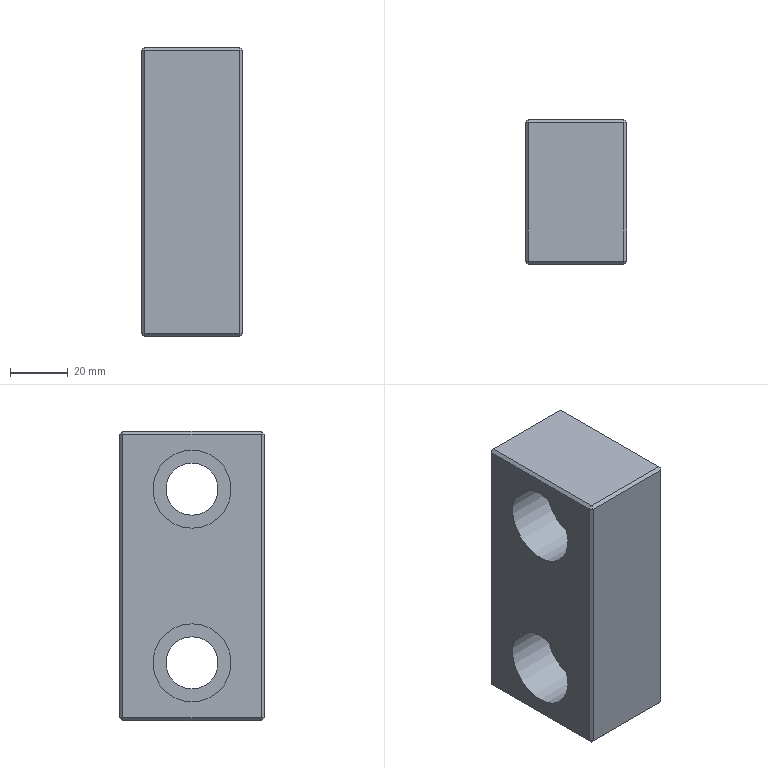Part | STEP file | 车灯-后视镜_id70_x_t | 1 solid | 32 faces | box 35 x 50 x 100 mm | volume 146008 mm3 | plane 28 | cylinder 4 | commonest cylinder face diameters 18 x2 27 x2
STEP:
#1=CARTESIAN_POINT('',(-284.,229.,49.5));
#2=VERTEX_POINT('',#1);
#3=CARTESIAN_POINT('',(-284.,181.,49.5));
#4=VERTEX_POINT('',#3);
#5=CARTESIAN_POINT('',(-284.,205.,49.5));
#6=DIRECTION('',(0.,-1.,0.));
#7=VECTOR('',#6,1.);
#8=LINE('',#5,#7);
#9=EDGE_CURVE('',#2,#4,#8,.T.);
#10=ORIENTED_EDGE('',*,*,#9,.T.);
#11=CARTESIAN_POINT('',(-251.,181.,49.5));
#12=VERTEX_POINT('',#11);
#13=CARTESIAN_POINT('',(-265.,181.,49.5));
#14=DIRECTION('',(1.,0.,0.));
#15=VECTOR('',#14,1.);
#16=LINE('',#13,#15);
#17=EDGE_CURVE('',#4,#12,#16,.T.);
#18=ORIENTED_EDGE('',*,*,#17,.T.);
#19=CARTESIAN_POINT('',(-251.,229.,49.5));
#20=VERTEX_POINT('',#19);
#21=CARTESIAN_POINT('',(-251.,205.,49.5));
#22=DIRECTION('',(0.,1.,0.));
#23=VECTOR('',#22,1.);
#24=LINE('',#21,#23);
#25=EDGE_CURVE('',#12,#20,#24,.T.);
#26=ORIENTED_EDGE('',*,*,#25,.T.);
#27=CARTESIAN_POINT('',(-265.,229.,49.5));
#28=DIRECTION('',(-1.,0.,0.));
#29=VECTOR('',#28,1.);
#30=LINE('',#27,#29);
#31=EDGE_CURVE('',#20,#2,#30,.T.);
#32=ORIENTED_EDGE('',*,*,#31,.T.);
#33=EDGE_LOOP('',(#10,#18,#26,#32));
#34=FACE_OUTER_BOUND('',#33,.T.);
#35=CARTESIAN_POINT('',(-265.,205.,49.5));
#36=DIRECTION('',(0.,0.,1.));
#37=DIRECTION('',(-1.,0.,0.));
#38=AXIS2_PLACEMENT_3D('',#35,#36,#37);
#39=PLANE('',#38);
#40=ADVANCED_FACE('',(#34),#39,.T.);
#41=CARTESIAN_POINT('',(-251.,230.,48.5));
#42=VERTEX_POINT('',#41);
#43=CARTESIAN_POINT('',(-251.,230.,-49.5));
#44=VERTEX_POINT('',#43);
#45=CARTESIAN_POINT('',(-251.,230.,-60.5));
#46=DIRECTION('',(0.,0.,-1.));
#47=VECTOR('',#46,1.);
#48=LINE('',#45,#47);
#49=EDGE_CURVE('',#42,#44,#48,.T.);
#50=ORIENTED_EDGE('',*,*,#49,.T.);
#51=CARTESIAN_POINT('',(-284.,230.,-49.5));
#52=VERTEX_POINT('',#51);
#53=CARTESIAN_POINT('',(-255.,230.,-49.5));
#54=DIRECTION('',(-1.,0.,0.));
#55=VECTOR('',#54,1.);
#56=LINE('',#53,#55);
#57=EDGE_CURVE('',#44,#52,#56,.T.);
#58=ORIENTED_EDGE('',*,*,#57,.T.);
#59=CARTESIAN_POINT('',(-284.,230.,48.5));
#60=VERTEX_POINT('',#59);
#61=CARTESIAN_POINT('',(-284.,230.,-60.5));
#62=DIRECTION('',(0.,0.,1.));
#63=VECTOR('',#62,1.);
#64=LINE('',#61,#63);
#65=EDGE_CURVE('',#52,#60,#64,.T.);
#66=ORIENTED_EDGE('',*,*,#65,.T.);
#67=CARTESIAN_POINT('',(-255.,230.,48.5));
#68=DIRECTION('',(1.,0.,0.));
#69=VECTOR('',#68,1.);
#70=LINE('',#67,#69);
#71=EDGE_CURVE('',#60,#42,#70,.T.);
#72=ORIENTED_EDGE('',*,*,#71,.T.);
#73=EDGE_LOOP('',(#50,#58,#66,#72));
#74=FACE_OUTER_BOUND('',#73,.T.);
#75=CARTESIAN_POINT('',(-255.,230.,-60.5));
#76=DIRECTION('',(0.,1.,0.));
#77=DIRECTION('',(0.,0.,-1.));
#78=AXIS2_PLACEMENT_3D('',#75,#76,#77);
#79=PLANE('',#78);
#80=ADVANCED_FACE('',(#74),#79,.T.);
#81=CARTESIAN_POINT('',(-250.,181.,48.5));
#82=VERTEX_POINT('',#81);
#83=CARTESIAN_POINT('',(-250.,181.,-49.5));
#84=VERTEX_POINT('',#83);
#85=CARTESIAN_POINT('',(-250.,181.,-60.5));
#86=DIRECTION('',(0.,0.,-1.));
#87=VECTOR('',#86,1.);
#88=LINE('',#85,#87);
#89=EDGE_CURVE('',#82,#84,#88,.T.);
#90=ORIENTED_EDGE('',*,*,#89,.T.);
#91=CARTESIAN_POINT('',(-250.,229.,-49.5));
#92=VERTEX_POINT('',#91);
#93=CARTESIAN_POINT('',(-250.,205.,-49.5));
#94=DIRECTION('',(0.,1.,0.));
#95=VECTOR('',#94,1.);
#96=LINE('',#93,#95);
#97=EDGE_CURVE('',#84,#92,#96,.T.);
#98=ORIENTED_EDGE('',*,*,#97,.T.);
#99=CARTESIAN_POINT('',(-250.,229.,48.5));
#100=VERTEX_POINT('',#99);
#101=CARTESIAN_POINT('',(-250.,229.,-60.5));
#102=DIRECTION('',(0.,0.,1.));
#103=VECTOR('',#102,1.);
#104=LINE('',#101,#103);
#105=EDGE_CURVE('',#92,#100,#104,.T.);
#106=ORIENTED_EDGE('',*,*,#105,.T.);
#107=CARTESIAN_POINT('',(-250.,205.,48.5));
#108=DIRECTION('',(0.,-1.,0.));
#109=VECTOR('',#108,1.);
#110=LINE('',#107,#109);
#111=EDGE_CURVE('',#100,#82,#110,.T.);
#112=ORIENTED_EDGE('',*,*,#111,.T.);
#113=EDGE_LOOP('',(#90,#98,#106,#112));
#114=FACE_BOUND('',#113,.T.);
#115=CARTESIAN_POINT('',(-250.,205.,-39.5));
#116=VERTEX_POINT('',#115);
#117=CARTESIAN_POINT('',(-250.,205.,-30.5));
#118=DIRECTION('',(-1.,0.,0.));
#119=DIRECTION('',(0.,0.,-1.));
#120=AXIS2_PLACEMENT_3D('',#117,#118,#119);
#121=CIRCLE('',#120,9.);
#122=EDGE_CURVE('',#116,#116,#121,.T.);
#123=ORIENTED_EDGE('',*,*,#122,.T.);
#124=EDGE_LOOP('',(#123));
#125=FACE_BOUND('',#124,.T.);
#126=CARTESIAN_POINT('',(-250.,205.,20.5));
#127=VERTEX_POINT('',#126);
#128=CARTESIAN_POINT('',(-250.,205.,29.5));
#129=DIRECTION('',(-1.,0.,0.));
#130=DIRECTION('',(0.,0.,-1.));
#131=AXIS2_PLACEMENT_3D('',#128,#129,#130);
#132=CIRCLE('',#131,9.);
#133=EDGE_CURVE('',#127,#127,#132,.T.);
#134=ORIENTED_EDGE('',*,*,#133,.T.);
#135=EDGE_LOOP('',(#134));
#136=FACE_BOUND('',#135,.T.);
#137=CARTESIAN_POINT('',(-250.,205.,-60.5));
#138=DIRECTION('',(1.,0.,0.));
#139=DIRECTION('',(0.,0.,1.));
#140=AXIS2_PLACEMENT_3D('',#137,#138,#139);
#141=PLANE('',#140);
#142=ADVANCED_FACE('',(#114,#125,#136),#141,.T.);
#143=CARTESIAN_POINT('',(-284.,180.,48.5));
#144=VERTEX_POINT('',#143);
#145=CARTESIAN_POINT('',(-284.,180.,-49.5));
#146=VERTEX_POINT('',#145);
#147=CARTESIAN_POINT('',(-284.,180.,-60.5));
#148=DIRECTION('',(0.,0.,-1.));
#149=VECTOR('',#148,1.);
#150=LINE('',#147,#149);
#151=EDGE_CURVE('',#144,#146,#150,.T.);
#152=ORIENTED_EDGE('',*,*,#151,.T.);
#153=CARTESIAN_POINT('',(-251.,180.,-49.5));
#154=VERTEX_POINT('',#153);
#155=CARTESIAN_POINT('',(-255.,180.,-49.5));
#156=DIRECTION('',(1.,0.,0.));
#157=VECTOR('',#156,1.);
#158=LINE('',#155,#157);
#159=EDGE_CURVE('',#146,#154,#158,.T.);
#160=ORIENTED_EDGE('',*,*,#159,.T.);
#161=CARTESIAN_POINT('',(-251.,180.,48.5));
#162=VERTEX_POINT('',#161);
#163=CARTESIAN_POINT('',(-251.,180.,-60.5));
#164=DIRECTION('',(0.,0.,1.));
#165=VECTOR('',#164,1.);
#166=LINE('',#163,#165);
#167=EDGE_CURVE('',#154,#162,#166,.T.);
#168=ORIENTED_EDGE('',*,*,#167,.T.);
#169=CARTESIAN_POINT('',(-255.,180.,48.5));
#170=DIRECTION('',(-1.,0.,0.));
#171=VECTOR('',#170,1.);
#172=LINE('',#169,#171);
#173=EDGE_CURVE('',#162,#144,#172,.T.);
#174=ORIENTED_EDGE('',*,*,#173,.T.);
#175=EDGE_LOOP('',(#152,#160,#168,#174));
#176=FACE_OUTER_BOUND('',#175,.T.);
#177=CARTESIAN_POINT('',(-255.,180.,-60.5));
#178=DIRECTION('',(0.,-1.,0.));
#179=DIRECTION('',(0.,0.,1.));
#180=AXIS2_PLACEMENT_3D('',#177,#178,#179);
#181=PLANE('',#180);
#182=ADVANCED_FACE('',(#176),#181,.T.);
#183=CARTESIAN_POINT('',(-284.,181.,-50.5));
#184=VERTEX_POINT('',#183);
#185=CARTESIAN_POINT('',(-284.,229.,-50.5));
#186=VERTEX_POINT('',#185);
#187=CARTESIAN_POINT('',(-284.,205.,-50.5));
#188=DIRECTION('',(0.,1.,0.));
#189=VECTOR('',#188,1.);
#190=LINE('',#187,#189);
#191=EDGE_CURVE('',#184,#186,#190,.T.);
#192=ORIENTED_EDGE('',*,*,#191,.T.);
#193=CARTESIAN_POINT('',(-251.,229.,-50.5));
#194=VERTEX_POINT('',#193);
#195=CARTESIAN_POINT('',(-265.,229.,-50.5));
#196=DIRECTION('',(1.,0.,0.));
#197=VECTOR('',#196,1.);
#198=LINE('',#195,#197);
#199=EDGE_CURVE('',#186,#194,#198,.T.);
#200=ORIENTED_EDGE('',*,*,#199,.T.);
#201=CARTESIAN_POINT('',(-251.,181.,-50.5));
#202=VERTEX_POINT('',#201);
#203=CARTESIAN_POINT('',(-251.,205.,-50.5));
#204=DIRECTION('',(0.,-1.,0.));
#205=VECTOR('',#204,1.);
#206=LINE('',#203,#205);
#207=EDGE_CURVE('',#194,#202,#206,.T.);
#208=ORIENTED_EDGE('',*,*,#207,.T.);
#209=CARTESIAN_POINT('',(-265.,181.,-50.5));
#210=DIRECTION('',(-1.,0.,0.));
#211=VECTOR('',#210,1.);
#212=LINE('',#209,#211);
#213=EDGE_CURVE('',#202,#184,#212,.T.);
#214=ORIENTED_EDGE('',*,*,#213,.T.);
#215=EDGE_LOOP('',(#192,#200,#208,#214));
#216=FACE_OUTER_BOUND('',#215,.T.);
#217=CARTESIAN_POINT('',(-265.,205.,-50.5));
#218=DIRECTION('',(0.,0.,-1.));
#219=DIRECTION('',(1.,0.,0.));
#220=AXIS2_PLACEMENT_3D('',#217,#218,#219);
#221=PLANE('',#220);
#222=ADVANCED_FACE('',(#216),#221,.T.);
#223=CARTESIAN_POINT('',(-285.,229.,48.5));
#224=VERTEX_POINT('',#223);
#225=CARTESIAN_POINT('',(-285.,229.,-49.5));
#226=VERTEX_POINT('',#225);
#227=CARTESIAN_POINT('',(-285.,229.,-60.5));
#228=DIRECTION('',(0.,0.,-1.));
#229=VECTOR('',#228,1.);
#230=LINE('',#227,#229);
#231=EDGE_CURVE('',#224,#226,#230,.T.);
#232=ORIENTED_EDGE('',*,*,#231,.T.);
#233=CARTESIAN_POINT('',(-285.,181.,-49.5));
#234=VERTEX_POINT('',#233);
#235=CARTESIAN_POINT('',(-285.,205.,-49.5));
#236=DIRECTION('',(0.,-1.,0.));
#237=VECTOR('',#236,1.);
#238=LINE('',#235,#237);
#239=EDGE_CURVE('',#226,#234,#238,.T.);
#240=ORIENTED_EDGE('',*,*,#239,.T.);
#241=CARTESIAN_POINT('',(-285.,181.,48.5));
#242=VERTEX_POINT('',#241);
#243=CARTESIAN_POINT('',(-285.,181.,-60.5));
#244=DIRECTION('',(0.,0.,1.));
#245=VECTOR('',#244,1.);
#246=LINE('',#243,#245);
#247=EDGE_CURVE('',#234,#242,#246,.T.);
#248=ORIENTED_EDGE('',*,*,#247,.T.);
#249=CARTESIAN_POINT('',(-285.,205.,48.5));
#250=DIRECTION('',(0.,1.,0.));
#251=VECTOR('',#250,1.);
#252=LINE('',#249,#251);
#253=EDGE_CURVE('',#242,#224,#252,.T.);
#254=ORIENTED_EDGE('',*,*,#253,.T.);
#255=EDGE_LOOP('',(#232,#240,#248,#254));
#256=FACE_BOUND('',#255,.T.);
#257=CARTESIAN_POINT('',(-285.,205.,-44.));
#258=VERTEX_POINT('',#257);
#259=CARTESIAN_POINT('',(-285.,205.,-30.5));
#260=DIRECTION('',(1.,0.,0.));
#261=DIRECTION('',(0.,0.,-1.));
#262=AXIS2_PLACEMENT_3D('',#259,#260,#261);
#263=CIRCLE('',#262,13.5);
#264=EDGE_CURVE('',#258,#258,#263,.T.);
#265=ORIENTED_EDGE('',*,*,#264,.T.);
#266=EDGE_LOOP('',(#265));
#267=FACE_BOUND('',#266,.T.);
#268=CARTESIAN_POINT('',(-285.,205.,16.));
#269=VERTEX_POINT('',#268);
#270=CARTESIAN_POINT('',(-285.,205.,29.5));
#271=DIRECTION('',(1.,0.,0.));
#272=DIRECTION('',(0.,0.,-1.));
#273=AXIS2_PLACEMENT_3D('',#270,#271,#272);
#274=CIRCLE('',#273,13.5);
#275=EDGE_CURVE('',#269,#269,#274,.T.);
#276=ORIENTED_EDGE('',*,*,#275,.T.);
#277=EDGE_LOOP('',(#276));
#278=FACE_BOUND('',#277,.T.);
#279=CARTESIAN_POINT('',(-285.,205.,-60.5));
#280=DIRECTION('',(-1.,0.,0.));
#281=DIRECTION('',(0.,0.,-1.));
#282=AXIS2_PLACEMENT_3D('',#279,#280,#281);
#283=PLANE('',#282);
#284=ADVANCED_FACE('',(#256,#267,#278),#283,.T.);
#285=CARTESIAN_POINT('',(-268.,205.,20.5));
#286=VERTEX_POINT('',#285);
#287=CARTESIAN_POINT('',(-268.,205.,29.5));
#288=DIRECTION('',(-1.,0.,0.));
#289=DIRECTION('',(0.,0.,-1.));
#290=AXIS2_PLACEMENT_3D('',#287,#288,#289);
#291=CIRCLE('',#290,9.);
#292=EDGE_CURVE('',#286,#286,#291,.T.);
#293=ORIENTED_EDGE('',*,*,#292,.T.);
#294=EDGE_LOOP('',(#293));
#295=FACE_BOUND('',#294,.T.);
#296=ORIENTED_EDGE('',*,*,#133,.F.);
#297=EDGE_LOOP('',(#296));
#298=FACE_BOUND('',#297,.T.);
#299=CARTESIAN_POINT('',(-250.,205.,29.5));
#300=DIRECTION('',(-1.,0.,0.));
#301=DIRECTION('',(0.,0.,-1.));
#302=AXIS2_PLACEMENT_3D('',#299,#300,#301);
#303=CYLINDRICAL_SURFACE('',#302,9.);
#304=ADVANCED_FACE('',(#295,#298),#303,.F.);
#305=CARTESIAN_POINT('',(-268.,205.,-39.5));
#306=VERTEX_POINT('',#305);
#307=CARTESIAN_POINT('',(-268.,205.,-30.5));
#308=DIRECTION('',(-1.,0.,0.));
#309=DIRECTION('',(0.,0.,-1.));
#310=AXIS2_PLACEMENT_3D('',#307,#308,#309);
#311=CIRCLE('',#310,9.);
#312=EDGE_CURVE('',#306,#306,#311,.T.);
#313=ORIENTED_EDGE('',*,*,#312,.T.);
#314=EDGE_LOOP('',(#313));
#315=FACE_BOUND('',#314,.T.);
#316=ORIENTED_EDGE('',*,*,#122,.F.);
#317=EDGE_LOOP('',(#316));
#318=FACE_BOUND('',#317,.T.);
#319=CARTESIAN_POINT('',(-250.,205.,-30.5));
#320=DIRECTION('',(-1.,0.,0.));
#321=DIRECTION('',(0.,0.,-1.));
#322=AXIS2_PLACEMENT_3D('',#319,#320,#321);
#323=CYLINDRICAL_SURFACE('',#322,9.);
#324=ADVANCED_FACE('',(#315,#318),#323,.F.);
#325=CARTESIAN_POINT('',(-268.,205.,43.));
#326=VERTEX_POINT('',#325);
#327=CARTESIAN_POINT('',(-268.,205.,29.5));
#328=DIRECTION('',(-1.,0.,0.));
#329=DIRECTION('',(0.,0.,1.));
#330=AXIS2_PLACEMENT_3D('',#327,#328,#329);
#331=CIRCLE('',#330,13.5);
#332=EDGE_CURVE('',#326,#326,#331,.T.);
#333=ORIENTED_EDGE('',*,*,#332,.T.);
#334=EDGE_LOOP('',(#333));
#335=FACE_BOUND('',#334,.T.);
#336=ORIENTED_EDGE('',*,*,#292,.F.);
#337=EDGE_LOOP('',(#336));
#338=FACE_BOUND('',#337,.T.);
#339=CARTESIAN_POINT('',(-268.,205.,29.5));
#340=DIRECTION('',(1.,0.,0.));
#341=DIRECTION('',(0.,0.,-1.));
#342=AXIS2_PLACEMENT_3D('',#339,#340,#341);
#343=PLANE('',#342);
#344=ADVANCED_FACE('',(#335,#338),#343,.F.);
#345=ORIENTED_EDGE('',*,*,#332,.F.);
#346=EDGE_LOOP('',(#345));
#347=FACE_BOUND('',#346,.T.);
#348=ORIENTED_EDGE('',*,*,#275,.F.);
#349=EDGE_LOOP('',(#348));
#350=FACE_BOUND('',#349,.T.);
#351=CARTESIAN_POINT('',(-285.,205.,29.5));
#352=DIRECTION('',(1.,0.,0.));
#353=DIRECTION('',(0.,0.,-1.));
#354=AXIS2_PLACEMENT_3D('',#351,#352,#353);
#355=CYLINDRICAL_SURFACE('',#354,13.5);
#356=ADVANCED_FACE('',(#347,#350),#355,.F.);
#357=CARTESIAN_POINT('',(-268.,205.,-17.));
#358=VERTEX_POINT('',#357);
#359=CARTESIAN_POINT('',(-268.,205.,-30.5));
#360=DIRECTION('',(-1.,0.,0.));
#361=DIRECTION('',(0.,0.,1.));
#362=AXIS2_PLACEMENT_3D('',#359,#360,#361);
#363=CIRCLE('',#362,13.5);
#364=EDGE_CURVE('',#358,#358,#363,.T.);
#365=ORIENTED_EDGE('',*,*,#364,.T.);
#366=EDGE_LOOP('',(#365));
#367=FACE_BOUND('',#366,.T.);
#368=ORIENTED_EDGE('',*,*,#312,.F.);
#369=EDGE_LOOP('',(#368));
#370=FACE_BOUND('',#369,.T.);
#371=CARTESIAN_POINT('',(-268.,205.,-30.5));
#372=DIRECTION('',(1.,0.,0.));
#373=DIRECTION('',(0.,0.,-1.));
#374=AXIS2_PLACEMENT_3D('',#371,#372,#373);
#375=PLANE('',#374);
#376=ADVANCED_FACE('',(#367,#370),#375,.F.);
#377=ORIENTED_EDGE('',*,*,#364,.F.);
#378=EDGE_LOOP('',(#377));
#379=FACE_BOUND('',#378,.T.);
#380=ORIENTED_EDGE('',*,*,#264,.F.);
#381=EDGE_LOOP('',(#380));
#382=FACE_BOUND('',#381,.T.);
#383=CARTESIAN_POINT('',(-285.,205.,-30.5));
#384=DIRECTION('',(1.,0.,0.));
#385=DIRECTION('',(0.,0.,-1.));
#386=AXIS2_PLACEMENT_3D('',#383,#384,#385);
#387=CYLINDRICAL_SURFACE('',#386,13.5);
#388=ADVANCED_FACE('',(#379,#382),#387,.F.);
#389=CARTESIAN_POINT('',(-284.,180.5,49.));
#390=DIRECTION('',(0.,0.7071,0.7071));
#391=VECTOR('',#390,1.);
#392=LINE('',#389,#391);
#393=EDGE_CURVE('',#144,#4,#392,.T.);
#394=ORIENTED_EDGE('',*,*,#393,.F.);
#395=ORIENTED_EDGE('',*,*,#173,.F.);
#396=CARTESIAN_POINT('',(-251.,180.,48.5));
#397=DIRECTION('',(0.,-0.7071,-0.7071));
#398=VECTOR('',#397,1.);
#399=LINE('',#396,#398);
#400=EDGE_CURVE('',#12,#162,#399,.T.);
#401=ORIENTED_EDGE('',*,*,#400,.F.);
#402=ORIENTED_EDGE('',*,*,#17,.F.);
#403=EDGE_LOOP('',(#394,#395,#401,#402));
#404=FACE_OUTER_BOUND('',#403,.T.);
#405=CARTESIAN_POINT('',(-265.,181.,49.5));
#406=DIRECTION('',(0.,0.7071,-0.7071));
#407=DIRECTION('',(0.,0.7071,0.7071));
#408=AXIS2_PLACEMENT_3D('',#405,#406,#407);
#409=PLANE('',#408);
#410=ADVANCED_FACE('',(#404),#409,.F.);
#411=CARTESIAN_POINT('',(-285.,181.,48.5));
#412=DIRECTION('',(-0.7071,0.7071,0.));
#413=VECTOR('',#412,1.);
#414=LINE('',#411,#413);
#415=EDGE_CURVE('',#144,#242,#414,.T.);
#416=ORIENTED_EDGE('',*,*,#415,.F.);
#417=ORIENTED_EDGE('',*,*,#393,.T.);
#418=CARTESIAN_POINT('',(-285.,181.,48.5));
#419=DIRECTION('',(0.7071,0.,0.7071));
#420=VECTOR('',#419,1.);
#421=LINE('',#418,#420);
#422=EDGE_CURVE('',#242,#4,#421,.T.);
#423=ORIENTED_EDGE('',*,*,#422,.F.);
#424=EDGE_LOOP('',(#416,#417,#423));
#425=FACE_OUTER_BOUND('',#424,.T.);
#426=CARTESIAN_POINT('',(-285.,181.,48.5));
#427=DIRECTION('',(-0.5774,-0.5774,0.5774));
#428=DIRECTION('',(0.7071,0.,0.7071));
#429=AXIS2_PLACEMENT_3D('',#426,#427,#428);
#430=PLANE('',#429);
#431=ADVANCED_FACE('',(#425),#430,.T.);
#432=CARTESIAN_POINT('',(-250.5,181.,49.));
#433=DIRECTION('',(0.7071,0.,-0.7071));
#434=VECTOR('',#433,1.);
#435=LINE('',#432,#434);
#436=EDGE_CURVE('',#12,#82,#435,.T.);
#437=ORIENTED_EDGE('',*,*,#436,.F.);
#438=ORIENTED_EDGE('',*,*,#400,.T.);
#439=CARTESIAN_POINT('',(-251.,180.,48.5));
#440=DIRECTION('',(-0.7071,-0.7071,0.));
#441=VECTOR('',#440,1.);
#442=LINE('',#439,#441);
#443=EDGE_CURVE('',#82,#162,#442,.T.);
#444=ORIENTED_EDGE('',*,*,#443,.F.);
#445=EDGE_LOOP('',(#437,#438,#444));
#446=FACE_OUTER_BOUND('',#445,.T.);
#447=CARTESIAN_POINT('',(-251.,180.,48.5));
#448=DIRECTION('',(0.5774,-0.5774,0.5774));
#449=DIRECTION('',(0.7071,0.,-0.7071));
#450=AXIS2_PLACEMENT_3D('',#447,#448,#449);
#451=PLANE('',#450);
#452=ADVANCED_FACE('',(#446),#451,.T.);
#453=ORIENTED_EDGE('',*,*,#422,.T.);
#454=ORIENTED_EDGE('',*,*,#9,.F.);
#455=CARTESIAN_POINT('',(-284.5,229.,49.));
#456=DIRECTION('',(0.7071,0.,0.7071));
#457=VECTOR('',#456,1.);
#458=LINE('',#455,#457);
#459=EDGE_CURVE('',#224,#2,#458,.T.);
#460=ORIENTED_EDGE('',*,*,#459,.F.);
#461=ORIENTED_EDGE('',*,*,#253,.F.);
#462=EDGE_LOOP('',(#453,#454,#460,#461));
#463=FACE_OUTER_BOUND('',#462,.T.);
#464=CARTESIAN_POINT('',(-285.,205.,48.5));
#465=DIRECTION('',(0.7071,0.,-0.7071));
#466=DIRECTION('',(-0.7071,0.,-0.7071));
#467=AXIS2_PLACEMENT_3D('',#464,#465,#466);
#468=PLANE('',#467);
#469=ADVANCED_FACE('',(#463),#468,.F.);
#470=ORIENTED_EDGE('',*,*,#415,.T.);
#471=ORIENTED_EDGE('',*,*,#247,.F.);
#472=CARTESIAN_POINT('',(-285.,181.,-49.5));
#473=DIRECTION('',(-0.7071,0.7071,0.));
#474=VECTOR('',#473,1.);
#475=LINE('',#472,#474);
#476=EDGE_CURVE('',#146,#234,#475,.T.);
#477=ORIENTED_EDGE('',*,*,#476,.F.);
#478=ORIENTED_EDGE('',*,*,#151,.F.);
#479=EDGE_LOOP('',(#470,#471,#477,#478));
#480=FACE_OUTER_BOUND('',#479,.T.);
#481=CARTESIAN_POINT('',(-285.,181.,-60.5));
#482=DIRECTION('',(0.7071,0.7071,0.));
#483=DIRECTION('',(-0.7071,0.7071,0.));
#484=AXIS2_PLACEMENT_3D('',#481,#482,#483);
#485=PLANE('',#484);
#486=ADVANCED_FACE('',(#480),#485,.F.);
#487=CARTESIAN_POINT('',(-251.,180.,-49.5));
#488=DIRECTION('',(0.,0.7071,-0.7071));
#489=VECTOR('',#488,1.);
#490=LINE('',#487,#489);
#491=EDGE_CURVE('',#154,#202,#490,.T.);
#492=ORIENTED_EDGE('',*,*,#491,.F.);
#493=ORIENTED_EDGE('',*,*,#159,.F.);
#494=CARTESIAN_POINT('',(-284.,180.5,-50.));
#495=DIRECTION('',(0.,-0.7071,0.7071));
#496=VECTOR('',#495,1.);
#497=LINE('',#494,#496);
#498=EDGE_CURVE('',#184,#146,#497,.T.);
#499=ORIENTED_EDGE('',*,*,#498,.F.);
#500=ORIENTED_EDGE('',*,*,#213,.F.);
#501=EDGE_LOOP('',(#492,#493,#499,#500));
#502=FACE_OUTER_BOUND('',#501,.T.);
#503=CARTESIAN_POINT('',(-265.,181.,-50.5));
#504=DIRECTION('',(0.,0.7071,0.7071));
#505=DIRECTION('',(0.,-0.7071,0.7071));
#506=AXIS2_PLACEMENT_3D('',#503,#504,#505);
#507=PLANE('',#506);
#508=ADVANCED_FACE('',(#502),#507,.F.);
#509=ORIENTED_EDGE('',*,*,#443,.T.);
#510=ORIENTED_EDGE('',*,*,#167,.F.);
#511=CARTESIAN_POINT('',(-251.,180.,-49.5));
#512=DIRECTION('',(-0.7071,-0.7071,0.));
#513=VECTOR('',#512,1.);
#514=LINE('',#511,#513);
#515=EDGE_CURVE('',#84,#154,#514,.T.);
#516=ORIENTED_EDGE('',*,*,#515,.F.);
#517=ORIENTED_EDGE('',*,*,#89,.F.);
#518=EDGE_LOOP('',(#509,#510,#516,#517));
#519=FACE_OUTER_BOUND('',#518,.T.);
#520=CARTESIAN_POINT('',(-251.,180.,-60.5));
#521=DIRECTION('',(-0.7071,0.7071,0.));
#522=DIRECTION('',(-0.7071,-0.7071,0.));
#523=AXIS2_PLACEMENT_3D('',#520,#521,#522);
#524=PLANE('',#523);
#525=ADVANCED_FACE('',(#519),#524,.F.);
#526=ORIENTED_EDGE('',*,*,#436,.T.);
#527=ORIENTED_EDGE('',*,*,#111,.F.);
#528=CARTESIAN_POINT('',(-251.,229.,49.5));
#529=DIRECTION('',(0.7071,0.,-0.7071));
#530=VECTOR('',#529,1.);
#531=LINE('',#528,#530);
#532=EDGE_CURVE('',#20,#100,#531,.T.);
#533=ORIENTED_EDGE('',*,*,#532,.F.);
#534=ORIENTED_EDGE('',*,*,#25,.F.);
#535=EDGE_LOOP('',(#526,#527,#533,#534));
#536=FACE_OUTER_BOUND('',#535,.T.);
#537=CARTESIAN_POINT('',(-250.,205.,48.5));
#538=DIRECTION('',(-0.7071,0.,-0.7071));
#539=DIRECTION('',(-0.7071,0.,0.7071));
#540=AXIS2_PLACEMENT_3D('',#537,#538,#539);
#541=PLANE('',#540);
#542=ADVANCED_FACE('',(#536),#541,.F.);
#543=CARTESIAN_POINT('',(-284.,230.,48.5));
#544=DIRECTION('',(0.,0.7071,-0.7071));
#545=VECTOR('',#544,1.);
#546=LINE('',#543,#545);
#547=EDGE_CURVE('',#2,#60,#546,.T.);
#548=ORIENTED_EDGE('',*,*,#547,.F.);
#549=ORIENTED_EDGE('',*,*,#31,.F.);
#550=CARTESIAN_POINT('',(-251.,229.,49.5));
#551=DIRECTION('',(0.,-0.7071,0.7071));
#552=VECTOR('',#551,1.);
#553=LINE('',#550,#552);
#554=EDGE_CURVE('',#42,#20,#553,.T.);
#555=ORIENTED_EDGE('',*,*,#554,.F.);
#556=ORIENTED_EDGE('',*,*,#71,.F.);
#557=EDGE_LOOP('',(#548,#549,#555,#556));
#558=FACE_OUTER_BOUND('',#557,.T.);
#559=CARTESIAN_POINT('',(-265.,229.,49.5));
#560=DIRECTION('',(0.,-0.7071,-0.7071));
#561=DIRECTION('',(0.,0.7071,-0.7071));
#562=AXIS2_PLACEMENT_3D('',#559,#560,#561);
#563=PLANE('',#562);
#564=ADVANCED_FACE('',(#558),#563,.F.);
#565=ORIENTED_EDGE('',*,*,#459,.T.);
#566=ORIENTED_EDGE('',*,*,#547,.T.);
#567=CARTESIAN_POINT('',(-284.,230.,48.5));
#568=DIRECTION('',(0.7071,0.7071,0.));
#569=VECTOR('',#568,1.);
#570=LINE('',#567,#569);
#571=EDGE_CURVE('',#224,#60,#570,.T.);
#572=ORIENTED_EDGE('',*,*,#571,.F.);
#573=EDGE_LOOP('',(#565,#566,#572));
#574=FACE_OUTER_BOUND('',#573,.T.);
#575=CARTESIAN_POINT('',(-284.,230.,48.5));
#576=DIRECTION('',(-0.5774,0.5774,0.5774));
#577=DIRECTION('',(0.7071,0.,0.7071));
#578=AXIS2_PLACEMENT_3D('',#575,#576,#577);
#579=PLANE('',#578);
#580=ADVANCED_FACE('',(#574),#579,.T.);
#581=ORIENTED_EDGE('',*,*,#498,.T.);
#582=ORIENTED_EDGE('',*,*,#476,.T.);
#583=CARTESIAN_POINT('',(-285.,181.,-49.5));
#584=DIRECTION('',(-0.7071,0.,0.7071));
#585=VECTOR('',#584,1.);
#586=LINE('',#583,#585);
#587=EDGE_CURVE('',#184,#234,#586,.T.);
#588=ORIENTED_EDGE('',*,*,#587,.F.);
#589=EDGE_LOOP('',(#581,#582,#588));
#590=FACE_OUTER_BOUND('',#589,.T.);
#591=CARTESIAN_POINT('',(-285.,181.,-49.5));
#592=DIRECTION('',(-0.5774,-0.5774,-0.5774));
#593=DIRECTION('',(-0.7071,0.,0.7071));
#594=AXIS2_PLACEMENT_3D('',#591,#592,#593);
#595=PLANE('',#594);
#596=ADVANCED_FACE('',(#590),#595,.T.);
#597=ORIENTED_EDGE('',*,*,#515,.T.);
#598=ORIENTED_EDGE('',*,*,#491,.T.);
#599=CARTESIAN_POINT('',(-250.5,181.,-50.));
#600=DIRECTION('',(-0.7071,0.,-0.7071));
#601=VECTOR('',#600,1.);
#602=LINE('',#599,#601);
#603=EDGE_CURVE('',#84,#202,#602,.T.);
#604=ORIENTED_EDGE('',*,*,#603,.F.);
#605=EDGE_LOOP('',(#597,#598,#604));
#606=FACE_OUTER_BOUND('',#605,.T.);
#607=CARTESIAN_POINT('',(-251.,180.,-49.5));
#608=DIRECTION('',(0.5774,-0.5774,-0.5774));
#609=DIRECTION('',(-0.7071,0.,-0.7071));
#610=AXIS2_PLACEMENT_3D('',#607,#608,#609);
#611=PLANE('',#610);
#612=ADVANCED_FACE('',(#606),#611,.T.);
#613=ORIENTED_EDGE('',*,*,#554,.T.);
#614=ORIENTED_EDGE('',*,*,#532,.T.);
#615=CARTESIAN_POINT('',(-250.5,229.5,48.5));
#616=DIRECTION('',(0.7071,-0.7071,0.));
#617=VECTOR('',#616,1.);
#618=LINE('',#615,#617);
#619=EDGE_CURVE('',#42,#100,#618,.T.);
#620=ORIENTED_EDGE('',*,*,#619,.F.);
#621=EDGE_LOOP('',(#613,#614,#620));
#622=FACE_OUTER_BOUND('',#621,.T.);
#623=CARTESIAN_POINT('',(-251.,229.,49.5));
#624=DIRECTION('',(0.5774,0.5774,0.5774));
#625=DIRECTION('',(0.7071,0.,-0.7071));
#626=AXIS2_PLACEMENT_3D('',#623,#624,#625);
#627=PLANE('',#626);
#628=ADVANCED_FACE('',(#622),#627,.T.);
#629=ORIENTED_EDGE('',*,*,#571,.T.);
#630=ORIENTED_EDGE('',*,*,#65,.F.);
#631=CARTESIAN_POINT('',(-284.,230.,-49.5));
#632=DIRECTION('',(0.7071,0.7071,0.));
#633=VECTOR('',#632,1.);
#634=LINE('',#631,#633);
#635=EDGE_CURVE('',#226,#52,#634,.T.);
#636=ORIENTED_EDGE('',*,*,#635,.F.);
#637=ORIENTED_EDGE('',*,*,#231,.F.);
#638=EDGE_LOOP('',(#629,#630,#636,#637));
#639=FACE_OUTER_BOUND('',#638,.T.);
#640=CARTESIAN_POINT('',(-284.,230.,-60.5));
#641=DIRECTION('',(0.7071,-0.7071,0.));
#642=DIRECTION('',(0.7071,0.7071,0.));
#643=AXIS2_PLACEMENT_3D('',#640,#641,#642);
#644=PLANE('',#643);
#645=ADVANCED_FACE('',(#639),#644,.F.);
#646=ORIENTED_EDGE('',*,*,#587,.T.);
#647=ORIENTED_EDGE('',*,*,#239,.F.);
#648=CARTESIAN_POINT('',(-284.5,229.,-50.));
#649=DIRECTION('',(-0.7071,0.,0.7071));
#650=VECTOR('',#649,1.);
#651=LINE('',#648,#650);
#652=EDGE_CURVE('',#186,#226,#651,.T.);
#653=ORIENTED_EDGE('',*,*,#652,.F.);
#654=ORIENTED_EDGE('',*,*,#191,.F.);
#655=EDGE_LOOP('',(#646,#647,#653,#654));
#656=FACE_OUTER_BOUND('',#655,.T.);
#657=CARTESIAN_POINT('',(-285.,205.,-49.5));
#658=DIRECTION('',(0.7071,0.,0.7071));
#659=DIRECTION('',(0.7071,0.,-0.7071));
#660=AXIS2_PLACEMENT_3D('',#657,#658,#659);
#661=PLANE('',#660);
#662=ADVANCED_FACE('',(#656),#661,.F.);
#663=ORIENTED_EDGE('',*,*,#603,.T.);
#664=ORIENTED_EDGE('',*,*,#207,.F.);
#665=CARTESIAN_POINT('',(-251.,229.,-50.5));
#666=DIRECTION('',(-0.7071,0.,-0.7071));
#667=VECTOR('',#666,1.);
#668=LINE('',#665,#667);
#669=EDGE_CURVE('',#92,#194,#668,.T.);
#670=ORIENTED_EDGE('',*,*,#669,.F.);
#671=ORIENTED_EDGE('',*,*,#97,.F.);
#672=EDGE_LOOP('',(#663,#664,#670,#671));
#673=FACE_OUTER_BOUND('',#672,.T.);
#674=CARTESIAN_POINT('',(-250.,205.,-49.5));
#675=DIRECTION('',(-0.7071,0.,0.7071));
#676=DIRECTION('',(0.7071,0.,0.7071));
#677=AXIS2_PLACEMENT_3D('',#674,#675,#676);
#678=PLANE('',#677);
#679=ADVANCED_FACE('',(#673),#678,.F.);
#680=ORIENTED_EDGE('',*,*,#619,.T.);
#681=ORIENTED_EDGE('',*,*,#105,.F.);
#682=CARTESIAN_POINT('',(-250.5,229.5,-49.5));
#683=DIRECTION('',(0.7071,-0.7071,0.));
#684=VECTOR('',#683,1.);
#685=LINE('',#682,#684);
#686=EDGE_CURVE('',#44,#92,#685,.T.);
#687=ORIENTED_EDGE('',*,*,#686,.F.);
#688=ORIENTED_EDGE('',*,*,#49,.F.);
#689=EDGE_LOOP('',(#680,#681,#687,#688));
#690=FACE_OUTER_BOUND('',#689,.T.);
#691=CARTESIAN_POINT('',(-250.,229.,-60.5));
#692=DIRECTION('',(-0.7071,-0.7071,0.));
#693=DIRECTION('',(0.7071,-0.7071,0.));
#694=AXIS2_PLACEMENT_3D('',#691,#692,#693);
#695=PLANE('',#694);
#696=ADVANCED_FACE('',(#690),#695,.F.);
#697=ORIENTED_EDGE('',*,*,#652,.T.);
#698=ORIENTED_EDGE('',*,*,#635,.T.);
#699=CARTESIAN_POINT('',(-284.,230.,-49.5));
#700=DIRECTION('',(0.,0.7071,0.7071));
#701=VECTOR('',#700,1.);
#702=LINE('',#699,#701);
#703=EDGE_CURVE('',#186,#52,#702,.T.);
#704=ORIENTED_EDGE('',*,*,#703,.F.);
#705=EDGE_LOOP('',(#697,#698,#704));
#706=FACE_OUTER_BOUND('',#705,.T.);
#707=CARTESIAN_POINT('',(-284.,230.,-49.5));
#708=DIRECTION('',(-0.5774,0.5774,-0.5774));
#709=DIRECTION('',(-0.7071,0.,0.7071));
#710=AXIS2_PLACEMENT_3D('',#707,#708,#709);
#711=PLANE('',#710);
#712=ADVANCED_FACE('',(#706),#711,.T.);
#713=ORIENTED_EDGE('',*,*,#686,.T.);
#714=ORIENTED_EDGE('',*,*,#669,.T.);
#715=CARTESIAN_POINT('',(-251.,229.,-50.5));
#716=DIRECTION('',(0.,-0.7071,-0.7071));
#717=VECTOR('',#716,1.);
#718=LINE('',#715,#717);
#719=EDGE_CURVE('',#44,#194,#718,.T.);
#720=ORIENTED_EDGE('',*,*,#719,.F.);
#721=EDGE_LOOP('',(#713,#714,#720));
#722=FACE_OUTER_BOUND('',#721,.T.);
#723=CARTESIAN_POINT('',(-251.,229.,-50.5));
#724=DIRECTION('',(0.5774,0.5774,-0.5774));
#725=DIRECTION('',(-0.7071,0.,-0.7071));
#726=AXIS2_PLACEMENT_3D('',#723,#724,#725);
#727=PLANE('',#726);
#728=ADVANCED_FACE('',(#722),#727,.T.);
#729=ORIENTED_EDGE('',*,*,#703,.T.);
#730=ORIENTED_EDGE('',*,*,#57,.F.);
#731=ORIENTED_EDGE('',*,*,#719,.T.);
#732=ORIENTED_EDGE('',*,*,#199,.F.);
#733=EDGE_LOOP('',(#729,#730,#731,#732));
#734=FACE_OUTER_BOUND('',#733,.T.);
#735=CARTESIAN_POINT('',(-265.,229.,-50.5));
#736=DIRECTION('',(0.,-0.7071,0.7071));
#737=DIRECTION('',(0.,-0.7071,-0.7071));
#738=AXIS2_PLACEMENT_3D('',#735,#736,#737);
#739=PLANE('',#738);
#740=ADVANCED_FACE('',(#734),#739,.F.);
#741=CLOSED_SHELL('',(#40,#80,#142,#182,#222,#284,#304,#324,#344,#356,#376,#388,#410,#431,#452,#469,#486,#508,#525,#542,#564,#580,#596,#612,#628,#645,#662,#679,#696,#712,#728,#740));
#742=MANIFOLD_SOLID_BREP('',#741);
#743=(LENGTH_UNIT()NAMED_UNIT(*)SI_UNIT(.MILLI.,.METRE.));
#744=UNCERTAINTY_MEASURE_WITH_UNIT(LENGTH_MEASURE(0.00002),#743,'','');
#745=(NAMED_UNIT(*)PLANE_ANGLE_UNIT()SI_UNIT($,.RADIAN.));
#746=PLANE_ANGLE_MEASURE_WITH_UNIT(PLANE_ANGLE_MEASURE(0.01745),#745);
#747=DIMENSIONAL_EXPONENTS(0.,0.,0.,0.,0.,0.,0.);
#748=(CONVERSION_BASED_UNIT('DEGREE',#746)NAMED_UNIT(#747)PLANE_ANGLE_UNIT());
#749=(NAMED_UNIT(*)SI_UNIT($,.STERADIAN.)SOLID_ANGLE_UNIT());
#750=(GEOMETRIC_REPRESENTATION_CONTEXT(3)GLOBAL_UNCERTAINTY_ASSIGNED_CONTEXT((#744))GLOBAL_UNIT_ASSIGNED_CONTEXT((#743,#748,#749))REPRESENTATION_CONTEXT('',''));
#751=ADVANCED_BREP_SHAPE_REPRESENTATION('',(#742),#750);